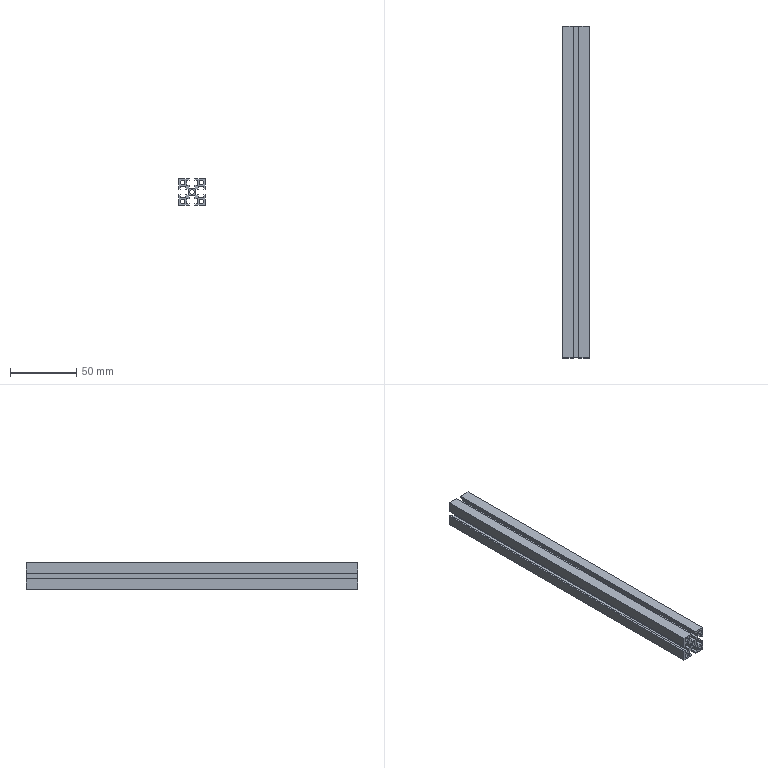Part | STEP file | 20 aluminium profile vertical 2 | 1 solid | 64 faces | box 20 x 250 x 20 mm | volume 44445 mm3 | plane 54 | cylinder 10 | commonest cylinder face diameters 3.3 x10